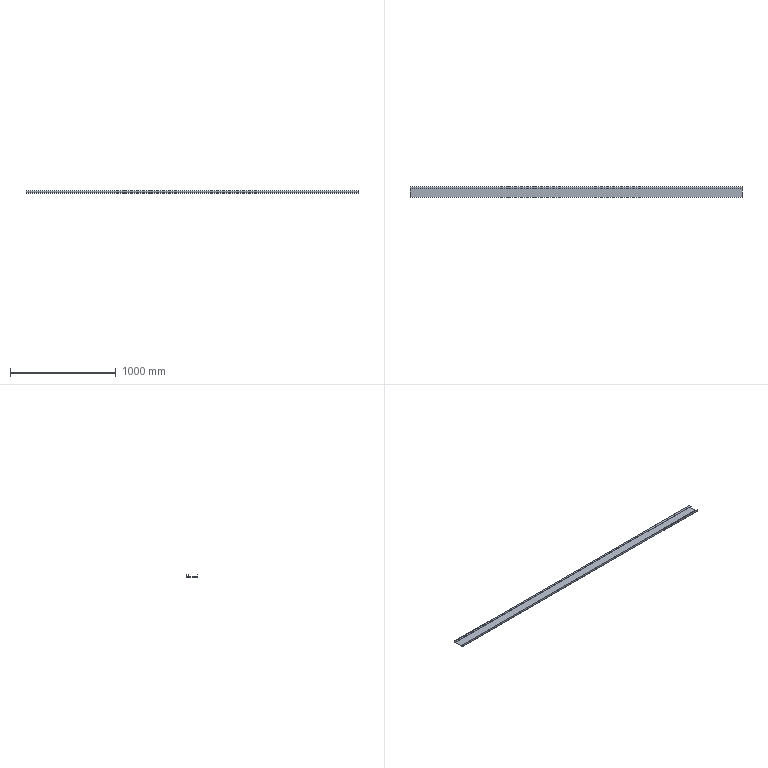Part | STEP file | 电柜护栏2踢脚Plate | 1 solid | 18 faces | box 3145 x 100 x 20 mm | volume 722941 mm3 | plane 12 | cylinder 6 | commonest cylinder face diameters 2 x3 5 x3
STEP:
#1=CARTESIAN_POINT('',(0.,0.,0.));
#2=DIRECTION('',(0.,0.,1.));
#3=DIRECTION('',(1.,0.,0.));
#4=AXIS2_PLACEMENT_3D('',#1,#2,#3);
#5=CARTESIAN_POINT('',(-1572.5,1.5,2.5));
#6=VERTEX_POINT('',#5);
#7=CARTESIAN_POINT('',(-1572.5,1.5,20.));
#8=VERTEX_POINT('',#7);
#9=CARTESIAN_POINT('',(-1572.5,1.5,2.5));
#10=DIRECTION('',(0.,0.,1.));
#11=VECTOR('',#10,1.);
#12=LINE('',#9,#11);
#13=CARTESIAN_POINT('',(1572.5,1.5,2.5));
#14=DIRECTION('',(0.,-1.,0.));
#15=DIRECTION('',(0.,0.,-1.));
#16=AXIS2_PLACEMENT_3D('',#13,#14,#15);
#17=PLANE('',#16);
#18=CARTESIAN_POINT('',(0.,-3145.));
#19=DIRECTION('',(-1.,0.));
#20=VECTOR('',#19,1.);
#21=LINE('',#18,#20);
#22=(GEOMETRIC_REPRESENTATION_CONTEXT(2)PARAMETRIC_REPRESENTATION_CONTEXT()REPRESENTATION_CONTEXT('',''));
#23=DEFINITIONAL_REPRESENTATION('',(#21),#22);
#24=PCURVE('',#17,#23);
#25=CARTESIAN_POINT('',(-1572.5,2.5,2.5));
#26=DIRECTION('',(-1.,0.,0.));
#27=DIRECTION('',(0.,0.,1.));
#28=AXIS2_PLACEMENT_3D('',#25,#26,#27);
#29=PLANE('',#28);
#30=CARTESIAN_POINT('',(0.,-1.));
#31=DIRECTION('',(1.,0.));
#32=VECTOR('',#31,1.);
#33=LINE('',#30,#32);
#34=(GEOMETRIC_REPRESENTATION_CONTEXT(2)PARAMETRIC_REPRESENTATION_CONTEXT()REPRESENTATION_CONTEXT('',''));
#35=DEFINITIONAL_REPRESENTATION('',(#33),#34);
#36=PCURVE('',#29,#35);
#37=SURFACE_CURVE('',#12,(#24,#36),.PCURVE_S1.);
#38=EDGE_CURVE('',#6,#8,#37,.T.);
#39=ORIENTED_EDGE('',*,*,#38,.T.);
#40=CARTESIAN_POINT('',(1572.5,1.5,20.));
#41=VERTEX_POINT('',#40);
#42=CARTESIAN_POINT('',(1572.5,1.5,20.));
#43=DIRECTION('',(-1.,0.,0.));
#44=VECTOR('',#43,1.);
#45=LINE('',#42,#44);
#46=CARTESIAN_POINT('',(-17.5,0.));
#47=DIRECTION('',(0.,-1.));
#48=VECTOR('',#47,1.);
#49=LINE('',#46,#48);
#50=(GEOMETRIC_REPRESENTATION_CONTEXT(2)PARAMETRIC_REPRESENTATION_CONTEXT()REPRESENTATION_CONTEXT('',''));
#51=DEFINITIONAL_REPRESENTATION('',(#49),#50);
#52=PCURVE('',#17,#51);
#53=CARTESIAN_POINT('',(1572.5,0.,20.));
#54=DIRECTION('',(0.,0.,1.));
#55=DIRECTION('',(1.,0.,0.));
#56=AXIS2_PLACEMENT_3D('',#53,#54,#55);
#57=PLANE('',#56);
#58=CARTESIAN_POINT('',(0.,1.5));
#59=DIRECTION('',(-1.,0.));
#60=VECTOR('',#59,1.);
#61=LINE('',#58,#60);
#62=(GEOMETRIC_REPRESENTATION_CONTEXT(2)PARAMETRIC_REPRESENTATION_CONTEXT()REPRESENTATION_CONTEXT('',''));
#63=DEFINITIONAL_REPRESENTATION('',(#61),#62);
#64=PCURVE('',#57,#63);
#65=SURFACE_CURVE('',#45,(#52,#64),.PCURVE_S1.);
#66=EDGE_CURVE('',#41,#8,#65,.T.);
#67=ORIENTED_EDGE('',*,*,#66,.F.);
#68=CARTESIAN_POINT('',(1572.5,1.5,2.5));
#69=VERTEX_POINT('',#68);
#70=CARTESIAN_POINT('',(1572.5,1.5,2.5));
#71=DIRECTION('',(0.,0.,1.));
#72=VECTOR('',#71,1.);
#73=LINE('',#70,#72);
#74=CARTESIAN_POINT('',(0.,0.));
#75=DIRECTION('',(-1.,0.));
#76=VECTOR('',#75,1.);
#77=LINE('',#74,#76);
#78=(GEOMETRIC_REPRESENTATION_CONTEXT(2)PARAMETRIC_REPRESENTATION_CONTEXT()REPRESENTATION_CONTEXT('',''));
#79=DEFINITIONAL_REPRESENTATION('',(#77),#78);
#80=PCURVE('',#17,#79);
#81=CARTESIAN_POINT('',(1572.5,2.5,2.5));
#82=DIRECTION('',(-1.,0.,0.));
#83=DIRECTION('',(0.,0.,1.));
#84=AXIS2_PLACEMENT_3D('',#81,#82,#83);
#85=PLANE('',#84);
#86=CARTESIAN_POINT('',(0.,-1.));
#87=DIRECTION('',(1.,0.));
#88=VECTOR('',#87,1.);
#89=LINE('',#86,#88);
#90=(GEOMETRIC_REPRESENTATION_CONTEXT(2)PARAMETRIC_REPRESENTATION_CONTEXT()REPRESENTATION_CONTEXT('',''));
#91=DEFINITIONAL_REPRESENTATION('',(#89),#90);
#92=PCURVE('',#85,#91);
#93=SURFACE_CURVE('',#73,(#80,#92),.PCURVE_S1.);
#94=EDGE_CURVE('',#69,#41,#93,.T.);
#95=ORIENTED_EDGE('',*,*,#94,.F.);
#96=CARTESIAN_POINT('',(1572.5,1.5,2.5));
#97=DIRECTION('',(-1.,0.,0.));
#98=VECTOR('',#97,1.);
#99=LINE('',#96,#98);
#100=CARTESIAN_POINT('',(0.,0.));
#101=DIRECTION('',(0.,-1.));
#102=VECTOR('',#101,1.);
#103=LINE('',#100,#102);
#104=(GEOMETRIC_REPRESENTATION_CONTEXT(2)PARAMETRIC_REPRESENTATION_CONTEXT()REPRESENTATION_CONTEXT('',''));
#105=DEFINITIONAL_REPRESENTATION('',(#103),#104);
#106=PCURVE('',#17,#105);
#107=CARTESIAN_POINT('',(1572.5,2.5,2.5));
#108=DIRECTION('',(-1.,0.,0.));
#109=DIRECTION('',(0.,0.,1.));
#110=AXIS2_PLACEMENT_3D('',#107,#108,#109);
#111=CYLINDRICAL_SURFACE('',#110,1.);
#112=CARTESIAN_POINT('',(4.712,0.));
#113=DIRECTION('',(0.,1.));
#114=VECTOR('',#113,1.);
#115=LINE('',#112,#114);
#116=(GEOMETRIC_REPRESENTATION_CONTEXT(2)PARAMETRIC_REPRESENTATION_CONTEXT()REPRESENTATION_CONTEXT('',''));
#117=DEFINITIONAL_REPRESENTATION('',(#115),#116);
#118=PCURVE('',#111,#117);
#119=SURFACE_CURVE('',#99,(#106,#118),.PCURVE_S1.);
#120=EDGE_CURVE('',#69,#6,#119,.T.);
#121=ORIENTED_EDGE('',*,*,#120,.T.);
#122=EDGE_LOOP('',(#39,#67,#95,#121));
#123=FACE_BOUND('',#122,.T.);
#124=ADVANCED_FACE('',(#123),#17,.F.);
#125=CARTESIAN_POINT('',(-1572.5,0.,20.));
#126=VERTEX_POINT('',#125);
#127=CARTESIAN_POINT('',(-1572.5,0.,20.));
#128=DIRECTION('',(0.,1.,0.));
#129=VECTOR('',#128,1.);
#130=LINE('',#127,#129);
#131=CARTESIAN_POINT('',(-3145.,0.));
#132=DIRECTION('',(0.,1.));
#133=VECTOR('',#132,1.);
#134=LINE('',#131,#133);
#135=(GEOMETRIC_REPRESENTATION_CONTEXT(2)PARAMETRIC_REPRESENTATION_CONTEXT()REPRESENTATION_CONTEXT('',''));
#136=DEFINITIONAL_REPRESENTATION('',(#134),#135);
#137=PCURVE('',#57,#136);
#138=CARTESIAN_POINT('',(17.5,-2.5));
#139=DIRECTION('',(0.,1.));
#140=VECTOR('',#139,1.);
#141=LINE('',#138,#140);
#142=(GEOMETRIC_REPRESENTATION_CONTEXT(2)PARAMETRIC_REPRESENTATION_CONTEXT()REPRESENTATION_CONTEXT('',''));
#143=DEFINITIONAL_REPRESENTATION('',(#141),#142);
#144=PCURVE('',#29,#143);
#145=SURFACE_CURVE('',#130,(#137,#144),.PCURVE_S1.);
#146=EDGE_CURVE('',#126,#8,#145,.T.);
#147=ORIENTED_EDGE('',*,*,#146,.F.);
#148=CARTESIAN_POINT('',(1572.5,0.,20.));
#149=VERTEX_POINT('',#148);
#150=CARTESIAN_POINT('',(1572.5,0.,20.));
#151=DIRECTION('',(-1.,0.,0.));
#152=VECTOR('',#151,1.);
#153=LINE('',#150,#152);
#154=CARTESIAN_POINT('',(0.,0.));
#155=DIRECTION('',(-1.,0.));
#156=VECTOR('',#155,1.);
#157=LINE('',#154,#156);
#158=(GEOMETRIC_REPRESENTATION_CONTEXT(2)PARAMETRIC_REPRESENTATION_CONTEXT()REPRESENTATION_CONTEXT('',''));
#159=DEFINITIONAL_REPRESENTATION('',(#157),#158);
#160=PCURVE('',#57,#159);
#161=CARTESIAN_POINT('',(1572.5,0.,2.5));
#162=DIRECTION('',(0.,-1.,0.));
#163=DIRECTION('',(0.,0.,-1.));
#164=AXIS2_PLACEMENT_3D('',#161,#162,#163);
#165=PLANE('',#164);
#166=CARTESIAN_POINT('',(-17.5,0.));
#167=DIRECTION('',(0.,-1.));
#168=VECTOR('',#167,1.);
#169=LINE('',#166,#168);
#170=(GEOMETRIC_REPRESENTATION_CONTEXT(2)PARAMETRIC_REPRESENTATION_CONTEXT()REPRESENTATION_CONTEXT('',''));
#171=DEFINITIONAL_REPRESENTATION('',(#169),#170);
#172=PCURVE('',#165,#171);
#173=SURFACE_CURVE('',#153,(#160,#172),.PCURVE_S1.);
#174=EDGE_CURVE('',#149,#126,#173,.T.);
#175=ORIENTED_EDGE('',*,*,#174,.F.);
#176=CARTESIAN_POINT('',(1572.5,0.,20.));
#177=DIRECTION('',(0.,1.,0.));
#178=VECTOR('',#177,1.);
#179=LINE('',#176,#178);
#180=CARTESIAN_POINT('',(0.,0.));
#181=DIRECTION('',(0.,1.));
#182=VECTOR('',#181,1.);
#183=LINE('',#180,#182);
#184=(GEOMETRIC_REPRESENTATION_CONTEXT(2)PARAMETRIC_REPRESENTATION_CONTEXT()REPRESENTATION_CONTEXT('',''));
#185=DEFINITIONAL_REPRESENTATION('',(#183),#184);
#186=PCURVE('',#57,#185);
#187=CARTESIAN_POINT('',(17.5,-2.5));
#188=DIRECTION('',(0.,1.));
#189=VECTOR('',#188,1.);
#190=LINE('',#187,#189);
#191=(GEOMETRIC_REPRESENTATION_CONTEXT(2)PARAMETRIC_REPRESENTATION_CONTEXT()REPRESENTATION_CONTEXT('',''));
#192=DEFINITIONAL_REPRESENTATION('',(#190),#191);
#193=PCURVE('',#85,#192);
#194=SURFACE_CURVE('',#179,(#186,#193),.PCURVE_S1.);
#195=EDGE_CURVE('',#149,#41,#194,.T.);
#196=ORIENTED_EDGE('',*,*,#195,.T.);
#197=ORIENTED_EDGE('',*,*,#66,.T.);
#198=EDGE_LOOP('',(#147,#175,#196,#197));
#199=FACE_BOUND('',#198,.T.);
#200=ADVANCED_FACE('',(#199),#57,.T.);
#201=CARTESIAN_POINT('',(-1572.5,0.,2.5));
#202=VERTEX_POINT('',#201);
#203=CARTESIAN_POINT('',(-1572.5,0.,2.5));
#204=DIRECTION('',(0.,0.,1.));
#205=VECTOR('',#204,1.);
#206=LINE('',#203,#205);
#207=CARTESIAN_POINT('',(0.,-3145.));
#208=DIRECTION('',(-1.,0.));
#209=VECTOR('',#208,1.);
#210=LINE('',#207,#209);
#211=(GEOMETRIC_REPRESENTATION_CONTEXT(2)PARAMETRIC_REPRESENTATION_CONTEXT()REPRESENTATION_CONTEXT('',''));
#212=DEFINITIONAL_REPRESENTATION('',(#210),#211);
#213=PCURVE('',#165,#212);
#214=CARTESIAN_POINT('',(0.,-2.5));
#215=DIRECTION('',(1.,0.));
#216=VECTOR('',#215,1.);
#217=LINE('',#214,#216);
#218=(GEOMETRIC_REPRESENTATION_CONTEXT(2)PARAMETRIC_REPRESENTATION_CONTEXT()REPRESENTATION_CONTEXT('',''));
#219=DEFINITIONAL_REPRESENTATION('',(#217),#218);
#220=PCURVE('',#29,#219);
#221=SURFACE_CURVE('',#206,(#213,#220),.PCURVE_S1.);
#222=EDGE_CURVE('',#202,#126,#221,.T.);
#223=ORIENTED_EDGE('',*,*,#222,.F.);
#224=CARTESIAN_POINT('',(1572.5,0.,2.5));
#225=VERTEX_POINT('',#224);
#226=CARTESIAN_POINT('',(1572.5,0.,2.5));
#227=DIRECTION('',(-1.,0.,0.));
#228=VECTOR('',#227,1.);
#229=LINE('',#226,#228);
#230=CARTESIAN_POINT('',(0.,0.));
#231=DIRECTION('',(0.,-1.));
#232=VECTOR('',#231,1.);
#233=LINE('',#230,#232);
#234=(GEOMETRIC_REPRESENTATION_CONTEXT(2)PARAMETRIC_REPRESENTATION_CONTEXT()REPRESENTATION_CONTEXT('',''));
#235=DEFINITIONAL_REPRESENTATION('',(#233),#234);
#236=PCURVE('',#165,#235);
#237=CARTESIAN_POINT('',(1572.5,2.5,2.5));
#238=DIRECTION('',(-1.,0.,0.));
#239=DIRECTION('',(0.,0.,1.));
#240=AXIS2_PLACEMENT_3D('',#237,#238,#239);
#241=CYLINDRICAL_SURFACE('',#240,2.5);
#242=CARTESIAN_POINT('',(4.712,0.));
#243=DIRECTION('',(0.,1.));
#244=VECTOR('',#243,1.);
#245=LINE('',#242,#244);
#246=(GEOMETRIC_REPRESENTATION_CONTEXT(2)PARAMETRIC_REPRESENTATION_CONTEXT()REPRESENTATION_CONTEXT('',''));
#247=DEFINITIONAL_REPRESENTATION('',(#245),#246);
#248=PCURVE('',#241,#247);
#249=SURFACE_CURVE('',#229,(#236,#248),.PCURVE_S1.);
#250=EDGE_CURVE('',#225,#202,#249,.T.);
#251=ORIENTED_EDGE('',*,*,#250,.F.);
#252=CARTESIAN_POINT('',(1572.5,0.,2.5));
#253=DIRECTION('',(0.,0.,1.));
#254=VECTOR('',#253,1.);
#255=LINE('',#252,#254);
#256=CARTESIAN_POINT('',(0.,0.));
#257=DIRECTION('',(-1.,0.));
#258=VECTOR('',#257,1.);
#259=LINE('',#256,#258);
#260=(GEOMETRIC_REPRESENTATION_CONTEXT(2)PARAMETRIC_REPRESENTATION_CONTEXT()REPRESENTATION_CONTEXT('',''));
#261=DEFINITIONAL_REPRESENTATION('',(#259),#260);
#262=PCURVE('',#165,#261);
#263=CARTESIAN_POINT('',(0.,-2.5));
#264=DIRECTION('',(1.,0.));
#265=VECTOR('',#264,1.);
#266=LINE('',#263,#265);
#267=(GEOMETRIC_REPRESENTATION_CONTEXT(2)PARAMETRIC_REPRESENTATION_CONTEXT()REPRESENTATION_CONTEXT('',''));
#268=DEFINITIONAL_REPRESENTATION('',(#266),#267);
#269=PCURVE('',#85,#268);
#270=SURFACE_CURVE('',#255,(#262,#269),.PCURVE_S1.);
#271=EDGE_CURVE('',#225,#149,#270,.T.);
#272=ORIENTED_EDGE('',*,*,#271,.T.);
#273=ORIENTED_EDGE('',*,*,#174,.T.);
#274=EDGE_LOOP('',(#223,#251,#272,#273));
#275=FACE_BOUND('',#274,.T.);
#276=ADVANCED_FACE('',(#275),#165,.T.);
#277=CARTESIAN_POINT('',(-1572.5,2.5,0.));
#278=VERTEX_POINT('',#277);
#279=CARTESIAN_POINT('',(-1572.5,2.5,2.5));
#280=DIRECTION('',(-1.,0.,0.));
#281=DIRECTION('',(0.,0.,1.));
#282=AXIS2_PLACEMENT_3D('',#279,#280,#281);
#283=CIRCLE('',#282,2.5);
#284=CARTESIAN_POINT('',(0.,3145.));
#285=DIRECTION('',(1.,0.));
#286=VECTOR('',#285,1.);
#287=LINE('',#284,#286);
#288=(GEOMETRIC_REPRESENTATION_CONTEXT(2)PARAMETRIC_REPRESENTATION_CONTEXT()REPRESENTATION_CONTEXT('',''));
#289=DEFINITIONAL_REPRESENTATION('',(#287),#288);
#290=PCURVE('',#241,#289);
#291=CARTESIAN_POINT('',(0.,0.));
#292=DIRECTION('',(1.,0.));
#293=AXIS2_PLACEMENT_2D('',#291,#292);
#294=CIRCLE('',#293,2.5);
#295=(GEOMETRIC_REPRESENTATION_CONTEXT(2)PARAMETRIC_REPRESENTATION_CONTEXT()REPRESENTATION_CONTEXT('',''));
#296=DEFINITIONAL_REPRESENTATION('',(#294),#295);
#297=PCURVE('',#29,#296);
#298=SURFACE_CURVE('',#283,(#290,#297),.PCURVE_S1.);
#299=EDGE_CURVE('',#278,#202,#298,.T.);
#300=ORIENTED_EDGE('',*,*,#299,.F.);
#301=CARTESIAN_POINT('',(1572.5,2.5,0.));
#302=VERTEX_POINT('',#301);
#303=CARTESIAN_POINT('',(1572.5,2.5,0.));
#304=DIRECTION('',(-1.,0.,0.));
#305=VECTOR('',#304,1.);
#306=LINE('',#303,#305);
#307=CARTESIAN_POINT('',(3.142,0.));
#308=DIRECTION('',(0.,1.));
#309=VECTOR('',#308,1.);
#310=LINE('',#307,#309);
#311=(GEOMETRIC_REPRESENTATION_CONTEXT(2)PARAMETRIC_REPRESENTATION_CONTEXT()REPRESENTATION_CONTEXT('',''));
#312=DEFINITIONAL_REPRESENTATION('',(#310),#311);
#313=PCURVE('',#241,#312);
#314=CARTESIAN_POINT('',(1572.5,2.5,0.));
#315=DIRECTION('',(0.,0.,-1.));
#316=DIRECTION('',(-1.,0.,0.));
#317=AXIS2_PLACEMENT_3D('',#314,#315,#316);
#318=PLANE('',#317);
#319=CARTESIAN_POINT('',(0.,0.));
#320=DIRECTION('',(1.,0.));
#321=VECTOR('',#320,1.);
#322=LINE('',#319,#321);
#323=(GEOMETRIC_REPRESENTATION_CONTEXT(2)PARAMETRIC_REPRESENTATION_CONTEXT()REPRESENTATION_CONTEXT('',''));
#324=DEFINITIONAL_REPRESENTATION('',(#322),#323);
#325=PCURVE('',#318,#324);
#326=SURFACE_CURVE('',#306,(#313,#325),.PCURVE_S1.);
#327=EDGE_CURVE('',#302,#278,#326,.T.);
#328=ORIENTED_EDGE('',*,*,#327,.F.);
#329=CARTESIAN_POINT('',(1572.5,2.5,2.5));
#330=DIRECTION('',(-1.,0.,0.));
#331=DIRECTION('',(0.,0.,1.));
#332=AXIS2_PLACEMENT_3D('',#329,#330,#331);
#333=CIRCLE('',#332,2.5);
#334=CARTESIAN_POINT('',(0.,0.));
#335=DIRECTION('',(1.,0.));
#336=VECTOR('',#335,1.);
#337=LINE('',#334,#336);
#338=(GEOMETRIC_REPRESENTATION_CONTEXT(2)PARAMETRIC_REPRESENTATION_CONTEXT()REPRESENTATION_CONTEXT('',''));
#339=DEFINITIONAL_REPRESENTATION('',(#337),#338);
#340=PCURVE('',#241,#339);
#341=CARTESIAN_POINT('',(0.,0.));
#342=DIRECTION('',(1.,0.));
#343=AXIS2_PLACEMENT_2D('',#341,#342);
#344=CIRCLE('',#343,2.5);
#345=(GEOMETRIC_REPRESENTATION_CONTEXT(2)PARAMETRIC_REPRESENTATION_CONTEXT()REPRESENTATION_CONTEXT('',''));
#346=DEFINITIONAL_REPRESENTATION('',(#344),#345);
#347=PCURVE('',#85,#346);
#348=SURFACE_CURVE('',#333,(#340,#347),.PCURVE_S1.);
#349=EDGE_CURVE('',#302,#225,#348,.T.);
#350=ORIENTED_EDGE('',*,*,#349,.T.);
#351=ORIENTED_EDGE('',*,*,#250,.T.);
#352=EDGE_LOOP('',(#300,#328,#350,#351));
#353=FACE_BOUND('',#352,.T.);
#354=ADVANCED_FACE('',(#353),#241,.T.);
#355=CARTESIAN_POINT('',(-1572.5,97.5,0.));
#356=VERTEX_POINT('',#355);
#357=CARTESIAN_POINT('',(-1572.5,2.5,0.));
#358=DIRECTION('',(0.,-1.,0.));
#359=VECTOR('',#358,1.);
#360=LINE('',#357,#359);
#361=CARTESIAN_POINT('',(3145.,0.));
#362=DIRECTION('',(0.,-1.));
#363=VECTOR('',#362,1.);
#364=LINE('',#361,#363);
#365=(GEOMETRIC_REPRESENTATION_CONTEXT(2)PARAMETRIC_REPRESENTATION_CONTEXT()REPRESENTATION_CONTEXT('',''));
#366=DEFINITIONAL_REPRESENTATION('',(#364),#365);
#367=PCURVE('',#318,#366);
#368=CARTESIAN_POINT('',(-2.5,0.));
#369=DIRECTION('',(0.,-1.));
#370=VECTOR('',#369,1.);
#371=LINE('',#368,#370);
#372=(GEOMETRIC_REPRESENTATION_CONTEXT(2)PARAMETRIC_REPRESENTATION_CONTEXT()REPRESENTATION_CONTEXT('',''));
#373=DEFINITIONAL_REPRESENTATION('',(#371),#372);
#374=PCURVE('',#29,#373);
#375=SURFACE_CURVE('',#360,(#367,#374),.PCURVE_S1.);
#376=EDGE_CURVE('',#356,#278,#375,.T.);
#377=ORIENTED_EDGE('',*,*,#376,.F.);
#378=CARTESIAN_POINT('',(1572.5,97.5,0.));
#379=VERTEX_POINT('',#378);
#380=CARTESIAN_POINT('',(1572.5,97.5,0.));
#381=DIRECTION('',(-1.,0.,0.));
#382=VECTOR('',#381,1.);
#383=LINE('',#380,#382);
#384=CARTESIAN_POINT('',(0.,95.));
#385=DIRECTION('',(1.,0.));
#386=VECTOR('',#385,1.);
#387=LINE('',#384,#386);
#388=(GEOMETRIC_REPRESENTATION_CONTEXT(2)PARAMETRIC_REPRESENTATION_CONTEXT()REPRESENTATION_CONTEXT('',''));
#389=DEFINITIONAL_REPRESENTATION('',(#387),#388);
#390=PCURVE('',#318,#389);
#391=CARTESIAN_POINT('',(1572.5,97.5,2.5));
#392=DIRECTION('',(-1.,0.,0.));
#393=DIRECTION('',(0.,0.,1.));
#394=AXIS2_PLACEMENT_3D('',#391,#392,#393);
#395=CYLINDRICAL_SURFACE('',#394,2.5);
#396=CARTESIAN_POINT('',(3.142,0.));
#397=DIRECTION('',(0.,1.));
#398=VECTOR('',#397,1.);
#399=LINE('',#396,#398);
#400=(GEOMETRIC_REPRESENTATION_CONTEXT(2)PARAMETRIC_REPRESENTATION_CONTEXT()REPRESENTATION_CONTEXT('',''));
#401=DEFINITIONAL_REPRESENTATION('',(#399),#400);
#402=PCURVE('',#395,#401);
#403=SURFACE_CURVE('',#383,(#390,#402),.PCURVE_S1.);
#404=EDGE_CURVE('',#379,#356,#403,.T.);
#405=ORIENTED_EDGE('',*,*,#404,.F.);
#406=CARTESIAN_POINT('',(1572.5,2.5,0.));
#407=DIRECTION('',(0.,-1.,0.));
#408=VECTOR('',#407,1.);
#409=LINE('',#406,#408);
#410=CARTESIAN_POINT('',(0.,0.));
#411=DIRECTION('',(0.,-1.));
#412=VECTOR('',#411,1.);
#413=LINE('',#410,#412);
#414=(GEOMETRIC_REPRESENTATION_CONTEXT(2)PARAMETRIC_REPRESENTATION_CONTEXT()REPRESENTATION_CONTEXT('',''));
#415=DEFINITIONAL_REPRESENTATION('',(#413),#414);
#416=PCURVE('',#318,#415);
#417=CARTESIAN_POINT('',(-2.5,0.));
#418=DIRECTION('',(0.,-1.));
#419=VECTOR('',#418,1.);
#420=LINE('',#417,#419);
#421=(GEOMETRIC_REPRESENTATION_CONTEXT(2)PARAMETRIC_REPRESENTATION_CONTEXT()REPRESENTATION_CONTEXT('',''));
#422=DEFINITIONAL_REPRESENTATION('',(#420),#421);
#423=PCURVE('',#85,#422);
#424=SURFACE_CURVE('',#409,(#416,#423),.PCURVE_S1.);
#425=EDGE_CURVE('',#379,#302,#424,.T.);
#426=ORIENTED_EDGE('',*,*,#425,.T.);
#427=ORIENTED_EDGE('',*,*,#327,.T.);
#428=EDGE_LOOP('',(#377,#405,#426,#427));
#429=FACE_BOUND('',#428,.T.);
#430=ADVANCED_FACE('',(#429),#318,.T.);
#431=CARTESIAN_POINT('',(-1572.5,100.,2.5));
#432=VERTEX_POINT('',#431);
#433=CARTESIAN_POINT('',(-1572.5,97.5,2.5));
#434=DIRECTION('',(-1.,0.,0.));
#435=DIRECTION('',(0.,0.,-1.));
#436=AXIS2_PLACEMENT_3D('',#433,#434,#435);
#437=CIRCLE('',#436,2.5);
#438=CARTESIAN_POINT('',(-3.142,3145.));
#439=DIRECTION('',(1.,0.));
#440=VECTOR('',#439,1.);
#441=LINE('',#438,#440);
#442=(GEOMETRIC_REPRESENTATION_CONTEXT(2)PARAMETRIC_REPRESENTATION_CONTEXT()REPRESENTATION_CONTEXT('',''));
#443=DEFINITIONAL_REPRESENTATION('',(#441),#442);
#444=PCURVE('',#395,#443);
#445=CARTESIAN_POINT('',(0.,95.));
#446=DIRECTION('',(-1.,0.));
#447=AXIS2_PLACEMENT_2D('',#445,#446);
#448=CIRCLE('',#447,2.5);
#449=(GEOMETRIC_REPRESENTATION_CONTEXT(2)PARAMETRIC_REPRESENTATION_CONTEXT()REPRESENTATION_CONTEXT('',''));
#450=DEFINITIONAL_REPRESENTATION('',(#448),#449);
#451=PCURVE('',#29,#450);
#452=SURFACE_CURVE('',#437,(#444,#451),.PCURVE_S1.);
#453=EDGE_CURVE('',#432,#356,#452,.T.);
#454=ORIENTED_EDGE('',*,*,#453,.F.);
#455=CARTESIAN_POINT('',(1572.5,100.,2.5));
#456=VERTEX_POINT('',#455);
#457=CARTESIAN_POINT('',(1572.5,100.,2.5));
#458=DIRECTION('',(-1.,0.,0.));
#459=VECTOR('',#458,1.);
#460=LINE('',#457,#459);
#461=CARTESIAN_POINT('',(1.571,0.));
#462=DIRECTION('',(0.,1.));
#463=VECTOR('',#462,1.);
#464=LINE('',#461,#463);
#465=(GEOMETRIC_REPRESENTATION_CONTEXT(2)PARAMETRIC_REPRESENTATION_CONTEXT()REPRESENTATION_CONTEXT('',''));
#466=DEFINITIONAL_REPRESENTATION('',(#464),#465);
#467=PCURVE('',#395,#466);
#468=CARTESIAN_POINT('',(1572.5,100.,2.5));
#469=DIRECTION('',(0.,1.,0.));
#470=DIRECTION('',(0.,0.,1.));
#471=AXIS2_PLACEMENT_3D('',#468,#469,#470);
#472=PLANE('',#471);
#473=CARTESIAN_POINT('',(0.,0.));
#474=DIRECTION('',(0.,-1.));
#475=VECTOR('',#474,1.);
#476=LINE('',#473,#475);
#477=(GEOMETRIC_REPRESENTATION_CONTEXT(2)PARAMETRIC_REPRESENTATION_CONTEXT()REPRESENTATION_CONTEXT('',''));
#478=DEFINITIONAL_REPRESENTATION('',(#476),#477);
#479=PCURVE('',#472,#478);
#480=SURFACE_CURVE('',#460,(#467,#479),.PCURVE_S1.);
#481=EDGE_CURVE('',#456,#432,#480,.T.);
#482=ORIENTED_EDGE('',*,*,#481,.F.);
#483=CARTESIAN_POINT('',(1572.5,97.5,2.5));
#484=DIRECTION('',(-1.,0.,0.));
#485=DIRECTION('',(0.,0.,-1.));
#486=AXIS2_PLACEMENT_3D('',#483,#484,#485);
#487=CIRCLE('',#486,2.5);
#488=CARTESIAN_POINT('',(-3.142,0.));
#489=DIRECTION('',(1.,0.));
#490=VECTOR('',#489,1.);
#491=LINE('',#488,#490);
#492=(GEOMETRIC_REPRESENTATION_CONTEXT(2)PARAMETRIC_REPRESENTATION_CONTEXT()REPRESENTATION_CONTEXT('',''));
#493=DEFINITIONAL_REPRESENTATION('',(#491),#492);
#494=PCURVE('',#395,#493);
#495=CARTESIAN_POINT('',(0.,95.));
#496=DIRECTION('',(-1.,0.));
#497=AXIS2_PLACEMENT_2D('',#495,#496);
#498=CIRCLE('',#497,2.5);
#499=(GEOMETRIC_REPRESENTATION_CONTEXT(2)PARAMETRIC_REPRESENTATION_CONTEXT()REPRESENTATION_CONTEXT('',''));
#500=DEFINITIONAL_REPRESENTATION('',(#498),#499);
#501=PCURVE('',#85,#500);
#502=SURFACE_CURVE('',#487,(#494,#501),.PCURVE_S1.);
#503=EDGE_CURVE('',#456,#379,#502,.T.);
#504=ORIENTED_EDGE('',*,*,#503,.T.);
#505=ORIENTED_EDGE('',*,*,#404,.T.);
#506=EDGE_LOOP('',(#454,#482,#504,#505));
#507=FACE_BOUND('',#506,.T.);
#508=ADVANCED_FACE('',(#507),#395,.T.);
#509=CARTESIAN_POINT('',(-1572.5,100.,17.5));
#510=VERTEX_POINT('',#509);
#511=CARTESIAN_POINT('',(-1572.5,100.,2.5));
#512=DIRECTION('',(0.,0.,-1.));
#513=VECTOR('',#512,1.);
#514=LINE('',#511,#513);
#515=CARTESIAN_POINT('',(0.,-3145.));
#516=DIRECTION('',(-1.,0.));
#517=VECTOR('',#516,1.);
#518=LINE('',#515,#517);
#519=(GEOMETRIC_REPRESENTATION_CONTEXT(2)PARAMETRIC_REPRESENTATION_CONTEXT()REPRESENTATION_CONTEXT('',''));
#520=DEFINITIONAL_REPRESENTATION('',(#518),#519);
#521=PCURVE('',#472,#520);
#522=CARTESIAN_POINT('',(0.,97.5));
#523=DIRECTION('',(-1.,0.));
#524=VECTOR('',#523,1.);
#525=LINE('',#522,#524);
#526=(GEOMETRIC_REPRESENTATION_CONTEXT(2)PARAMETRIC_REPRESENTATION_CONTEXT()REPRESENTATION_CONTEXT('',''));
#527=DEFINITIONAL_REPRESENTATION('',(#525),#526);
#528=PCURVE('',#29,#527);
#529=SURFACE_CURVE('',#514,(#521,#528),.PCURVE_S1.);
#530=EDGE_CURVE('',#510,#432,#529,.T.);
#531=ORIENTED_EDGE('',*,*,#530,.F.);
#532=CARTESIAN_POINT('',(1572.5,100.,17.5));
#533=VERTEX_POINT('',#532);
#534=CARTESIAN_POINT('',(1572.5,100.,17.5));
#535=DIRECTION('',(-1.,0.,0.));
#536=VECTOR('',#535,1.);
#537=LINE('',#534,#536);
#538=CARTESIAN_POINT('',(15.,0.));
#539=DIRECTION('',(0.,-1.));
#540=VECTOR('',#539,1.);
#541=LINE('',#538,#540);
#542=(GEOMETRIC_REPRESENTATION_CONTEXT(2)PARAMETRIC_REPRESENTATION_CONTEXT()REPRESENTATION_CONTEXT('',''));
#543=DEFINITIONAL_REPRESENTATION('',(#541),#542);
#544=PCURVE('',#472,#543);
#545=CARTESIAN_POINT('',(1572.5,97.5,17.5));
#546=DIRECTION('',(-1.,0.,0.));
#547=DIRECTION('',(0.,0.,1.));
#548=AXIS2_PLACEMENT_3D('',#545,#546,#547);
#549=CYLINDRICAL_SURFACE('',#548,2.5);
#550=CARTESIAN_POINT('',(1.571,0.));
#551=DIRECTION('',(0.,1.));
#552=VECTOR('',#551,1.);
#553=LINE('',#550,#552);
#554=(GEOMETRIC_REPRESENTATION_CONTEXT(2)PARAMETRIC_REPRESENTATION_CONTEXT()REPRESENTATION_CONTEXT('',''));
#555=DEFINITIONAL_REPRESENTATION('',(#553),#554);
#556=PCURVE('',#549,#555);
#557=SURFACE_CURVE('',#537,(#544,#556),.PCURVE_S1.);
#558=EDGE_CURVE('',#533,#510,#557,.T.);
#559=ORIENTED_EDGE('',*,*,#558,.F.);
#560=CARTESIAN_POINT('',(1572.5,100.,2.5));
#561=DIRECTION('',(0.,0.,-1.));
#562=VECTOR('',#561,1.);
#563=LINE('',#560,#562);
#564=CARTESIAN_POINT('',(0.,0.));
#565=DIRECTION('',(-1.,0.));
#566=VECTOR('',#565,1.);
#567=LINE('',#564,#566);
#568=(GEOMETRIC_REPRESENTATION_CONTEXT(2)PARAMETRIC_REPRESENTATION_CONTEXT()REPRESENTATION_CONTEXT('',''));
#569=DEFINITIONAL_REPRESENTATION('',(#567),#568);
#570=PCURVE('',#472,#569);
#571=CARTESIAN_POINT('',(0.,97.5));
#572=DIRECTION('',(-1.,0.));
#573=VECTOR('',#572,1.);
#574=LINE('',#571,#573);
#575=(GEOMETRIC_REPRESENTATION_CONTEXT(2)PARAMETRIC_REPRESENTATION_CONTEXT()REPRESENTATION_CONTEXT('',''));
#576=DEFINITIONAL_REPRESENTATION('',(#574),#575);
#577=PCURVE('',#85,#576);
#578=SURFACE_CURVE('',#563,(#570,#577),.PCURVE_S1.);
#579=EDGE_CURVE('',#533,#456,#578,.T.);
#580=ORIENTED_EDGE('',*,*,#579,.T.);
#581=ORIENTED_EDGE('',*,*,#481,.T.);
#582=EDGE_LOOP('',(#531,#559,#580,#581));
#583=FACE_BOUND('',#582,.T.);
#584=ADVANCED_FACE('',(#583),#472,.T.);
#585=CARTESIAN_POINT('',(-1572.5,97.5,20.));
#586=VERTEX_POINT('',#585);
#587=CARTESIAN_POINT('',(-1572.5,97.5,17.5));
#588=DIRECTION('',(-1.,0.,0.));
#589=DIRECTION('',(0.,0.,-1.));
#590=AXIS2_PLACEMENT_3D('',#587,#588,#589);
#591=CIRCLE('',#590,2.5);
#592=CARTESIAN_POINT('',(-3.142,3145.));
#593=DIRECTION('',(1.,0.));
#594=VECTOR('',#593,1.);
#595=LINE('',#592,#594);
#596=(GEOMETRIC_REPRESENTATION_CONTEXT(2)PARAMETRIC_REPRESENTATION_CONTEXT()REPRESENTATION_CONTEXT('',''));
#597=DEFINITIONAL_REPRESENTATION('',(#595),#596);
#598=PCURVE('',#549,#597);
#599=CARTESIAN_POINT('',(15.,95.));
#600=DIRECTION('',(-1.,0.));
#601=AXIS2_PLACEMENT_2D('',#599,#600);
#602=CIRCLE('',#601,2.5);
#603=(GEOMETRIC_REPRESENTATION_CONTEXT(2)PARAMETRIC_REPRESENTATION_CONTEXT()REPRESENTATION_CONTEXT('',''));
#604=DEFINITIONAL_REPRESENTATION('',(#602),#603);
#605=PCURVE('',#29,#604);
#606=SURFACE_CURVE('',#591,(#598,#605),.PCURVE_S1.);
#607=EDGE_CURVE('',#586,#510,#606,.T.);
#608=ORIENTED_EDGE('',*,*,#607,.F.);
#609=CARTESIAN_POINT('',(1572.5,97.5,20.));
#610=VERTEX_POINT('',#609);
#611=CARTESIAN_POINT('',(1572.5,97.5,20.));
#612=DIRECTION('',(-1.,0.,0.));
#613=VECTOR('',#612,1.);
#614=LINE('',#611,#613);
#615=CARTESIAN_POINT('',(0.,0.));
#616=DIRECTION('',(0.,1.));
#617=VECTOR('',#616,1.);
#618=LINE('',#615,#617);
#619=(GEOMETRIC_REPRESENTATION_CONTEXT(2)PARAMETRIC_REPRESENTATION_CONTEXT()REPRESENTATION_CONTEXT('',''));
#620=DEFINITIONAL_REPRESENTATION('',(#618),#619);
#621=PCURVE('',#549,#620);
#622=CARTESIAN_POINT('',(1572.5,97.5,20.));
#623=DIRECTION('',(0.,0.,1.));
#624=DIRECTION('',(1.,0.,0.));
#625=AXIS2_PLACEMENT_3D('',#622,#623,#624);
#626=PLANE('',#625);
#627=CARTESIAN_POINT('',(0.,0.));
#628=DIRECTION('',(-1.,0.));
#629=VECTOR('',#628,1.);
#630=LINE('',#627,#629);
#631=(GEOMETRIC_REPRESENTATION_CONTEXT(2)PARAMETRIC_REPRESENTATION_CONTEXT()REPRESENTATION_CONTEXT('',''));
#632=DEFINITIONAL_REPRESENTATION('',(#630),#631);
#633=PCURVE('',#626,#632);
#634=SURFACE_CURVE('',#614,(#621,#633),.PCURVE_S1.);
#635=EDGE_CURVE('',#610,#586,#634,.T.);
#636=ORIENTED_EDGE('',*,*,#635,.F.);
#637=CARTESIAN_POINT('',(1572.5,97.5,17.5));
#638=DIRECTION('',(-1.,0.,0.));
#639=DIRECTION('',(0.,0.,-1.));
#640=AXIS2_PLACEMENT_3D('',#637,#638,#639);
#641=CIRCLE('',#640,2.5);
#642=CARTESIAN_POINT('',(-3.142,0.));
#643=DIRECTION('',(1.,0.));
#644=VECTOR('',#643,1.);
#645=LINE('',#642,#644);
#646=(GEOMETRIC_REPRESENTATION_CONTEXT(2)PARAMETRIC_REPRESENTATION_CONTEXT()REPRESENTATION_CONTEXT('',''));
#647=DEFINITIONAL_REPRESENTATION('',(#645),#646);
#648=PCURVE('',#549,#647);
#649=CARTESIAN_POINT('',(15.,95.));
#650=DIRECTION('',(-1.,0.));
#651=AXIS2_PLACEMENT_2D('',#649,#650);
#652=CIRCLE('',#651,2.5);
#653=(GEOMETRIC_REPRESENTATION_CONTEXT(2)PARAMETRIC_REPRESENTATION_CONTEXT()REPRESENTATION_CONTEXT('',''));
#654=DEFINITIONAL_REPRESENTATION('',(#652),#653);
#655=PCURVE('',#85,#654);
#656=SURFACE_CURVE('',#641,(#648,#655),.PCURVE_S1.);
#657=EDGE_CURVE('',#610,#533,#656,.T.);
#658=ORIENTED_EDGE('',*,*,#657,.T.);
#659=ORIENTED_EDGE('',*,*,#558,.T.);
#660=EDGE_LOOP('',(#608,#636,#658,#659));
#661=FACE_BOUND('',#660,.T.);
#662=ADVANCED_FACE('',(#661),#549,.T.);
#663=CARTESIAN_POINT('',(-1572.5,80.,20.));
#664=VERTEX_POINT('',#663);
#665=CARTESIAN_POINT('',(-1572.5,97.5,20.));
#666=DIRECTION('',(0.,1.,0.));
#667=VECTOR('',#666,1.);
#668=LINE('',#665,#667);
#669=CARTESIAN_POINT('',(-3145.,0.));
#670=DIRECTION('',(0.,1.));
#671=VECTOR('',#670,1.);
#672=LINE('',#669,#671);
#673=(GEOMETRIC_REPRESENTATION_CONTEXT(2)PARAMETRIC_REPRESENTATION_CONTEXT()REPRESENTATION_CONTEXT('',''));
#674=DEFINITIONAL_REPRESENTATION('',(#672),#673);
#675=PCURVE('',#626,#674);
#676=CARTESIAN_POINT('',(17.5,95.));
#677=DIRECTION('',(0.,1.));
#678=VECTOR('',#677,1.);
#679=LINE('',#676,#678);
#680=(GEOMETRIC_REPRESENTATION_CONTEXT(2)PARAMETRIC_REPRESENTATION_CONTEXT()REPRESENTATION_CONTEXT('',''));
#681=DEFINITIONAL_REPRESENTATION('',(#679),#680);
#682=PCURVE('',#29,#681);
#683=SURFACE_CURVE('',#668,(#675,#682),.PCURVE_S1.);
#684=EDGE_CURVE('',#664,#586,#683,.T.);
#685=ORIENTED_EDGE('',*,*,#684,.F.);
#686=CARTESIAN_POINT('',(1572.5,80.,20.));
#687=VERTEX_POINT('',#686);
#688=CARTESIAN_POINT('',(1572.5,80.,20.));
#689=DIRECTION('',(-1.,0.,0.));
#690=VECTOR('',#689,1.);
#691=LINE('',#688,#690);
#692=CARTESIAN_POINT('',(0.,-17.5));
#693=DIRECTION('',(-1.,0.));
#694=VECTOR('',#693,1.);
#695=LINE('',#692,#694);
#696=(GEOMETRIC_REPRESENTATION_CONTEXT(2)PARAMETRIC_REPRESENTATION_CONTEXT()REPRESENTATION_CONTEXT('',''));
#697=DEFINITIONAL_REPRESENTATION('',(#695),#696);
#698=PCURVE('',#626,#697);
#699=CARTESIAN_POINT('',(1572.5,80.,18.5));
#700=DIRECTION('',(0.,-1.,0.));
#701=DIRECTION('',(0.,0.,-1.));
#702=AXIS2_PLACEMENT_3D('',#699,#700,#701);
#703=PLANE('',#702);
#704=CARTESIAN_POINT('',(-1.5,0.));
#705=DIRECTION('',(0.,-1.));
#706=VECTOR('',#705,1.);
#707=LINE('',#704,#706);
#708=(GEOMETRIC_REPRESENTATION_CONTEXT(2)PARAMETRIC_REPRESENTATION_CONTEXT()REPRESENTATION_CONTEXT('',''));
#709=DEFINITIONAL_REPRESENTATION('',(#707),#708);
#710=PCURVE('',#703,#709);
#711=SURFACE_CURVE('',#691,(#698,#710),.PCURVE_S1.);
#712=EDGE_CURVE('',#687,#664,#711,.T.);
#713=ORIENTED_EDGE('',*,*,#712,.F.);
#714=CARTESIAN_POINT('',(1572.5,97.5,20.));
#715=DIRECTION('',(0.,1.,0.));
#716=VECTOR('',#715,1.);
#717=LINE('',#714,#716);
#718=CARTESIAN_POINT('',(0.,0.));
#719=DIRECTION('',(0.,1.));
#720=VECTOR('',#719,1.);
#721=LINE('',#718,#720);
#722=(GEOMETRIC_REPRESENTATION_CONTEXT(2)PARAMETRIC_REPRESENTATION_CONTEXT()REPRESENTATION_CONTEXT('',''));
#723=DEFINITIONAL_REPRESENTATION('',(#721),#722);
#724=PCURVE('',#626,#723);
#725=CARTESIAN_POINT('',(17.5,95.));
#726=DIRECTION('',(0.,1.));
#727=VECTOR('',#726,1.);
#728=LINE('',#725,#727);
#729=(GEOMETRIC_REPRESENTATION_CONTEXT(2)PARAMETRIC_REPRESENTATION_CONTEXT()REPRESENTATION_CONTEXT('',''));
#730=DEFINITIONAL_REPRESENTATION('',(#728),#729);
#731=PCURVE('',#85,#730);
#732=SURFACE_CURVE('',#717,(#724,#731),.PCURVE_S1.);
#733=EDGE_CURVE('',#687,#610,#732,.T.);
#734=ORIENTED_EDGE('',*,*,#733,.T.);
#735=ORIENTED_EDGE('',*,*,#635,.T.);
#736=EDGE_LOOP('',(#685,#713,#734,#735));
#737=FACE_BOUND('',#736,.T.);
#738=ADVANCED_FACE('',(#737),#626,.T.);
#739=CARTESIAN_POINT('',(-1572.5,80.,18.5));
#740=VERTEX_POINT('',#739);
#741=CARTESIAN_POINT('',(-1572.5,80.,18.5));
#742=DIRECTION('',(0.,0.,1.));
#743=VECTOR('',#742,1.);
#744=LINE('',#741,#743);
#745=CARTESIAN_POINT('',(0.,-3145.));
#746=DIRECTION('',(-1.,0.));
#747=VECTOR('',#746,1.);
#748=LINE('',#745,#747);
#749=(GEOMETRIC_REPRESENTATION_CONTEXT(2)PARAMETRIC_REPRESENTATION_CONTEXT()REPRESENTATION_CONTEXT('',''));
#750=DEFINITIONAL_REPRESENTATION('',(#748),#749);
#751=PCURVE('',#703,#750);
#752=CARTESIAN_POINT('',(16.,77.5));
#753=DIRECTION('',(1.,0.));
#754=VECTOR('',#753,1.);
#755=LINE('',#752,#754);
#756=(GEOMETRIC_REPRESENTATION_CONTEXT(2)PARAMETRIC_REPRESENTATION_CONTEXT()REPRESENTATION_CONTEXT('',''));
#757=DEFINITIONAL_REPRESENTATION('',(#755),#756);
#758=PCURVE('',#29,#757);
#759=SURFACE_CURVE('',#744,(#751,#758),.PCURVE_S1.);
#760=EDGE_CURVE('',#740,#664,#759,.T.);
#761=ORIENTED_EDGE('',*,*,#760,.F.);
#762=CARTESIAN_POINT('',(1572.5,80.,18.5));
#763=VERTEX_POINT('',#762);
#764=CARTESIAN_POINT('',(1572.5,80.,18.5));
#765=DIRECTION('',(-1.,0.,0.));
#766=VECTOR('',#765,1.);
#767=LINE('',#764,#766);
#768=CARTESIAN_POINT('',(0.,0.));
#769=DIRECTION('',(0.,-1.));
#770=VECTOR('',#769,1.);
#771=LINE('',#768,#770);
#772=(GEOMETRIC_REPRESENTATION_CONTEXT(2)PARAMETRIC_REPRESENTATION_CONTEXT()REPRESENTATION_CONTEXT('',''));
#773=DEFINITIONAL_REPRESENTATION('',(#771),#772);
#774=PCURVE('',#703,#773);
#775=CARTESIAN_POINT('',(1572.5,97.5,18.5));
#776=DIRECTION('',(0.,0.,1.));
#777=DIRECTION('',(1.,0.,0.));
#778=AXIS2_PLACEMENT_3D('',#775,#776,#777);
#779=PLANE('',#778);
#780=CARTESIAN_POINT('',(0.,-17.5));
#781=DIRECTION('',(-1.,0.));
#782=VECTOR('',#781,1.);
#783=LINE('',#780,#782);
#784=(GEOMETRIC_REPRESENTATION_CONTEXT(2)PARAMETRIC_REPRESENTATION_CONTEXT()REPRESENTATION_CONTEXT('',''));
#785=DEFINITIONAL_REPRESENTATION('',(#783),#784);
#786=PCURVE('',#779,#785);
#787=SURFACE_CURVE('',#767,(#774,#786),.PCURVE_S1.);
#788=EDGE_CURVE('',#763,#740,#787,.T.);
#789=ORIENTED_EDGE('',*,*,#788,.F.);
#790=CARTESIAN_POINT('',(1572.5,80.,18.5));
#791=DIRECTION('',(0.,0.,1.));
#792=VECTOR('',#791,1.);
#793=LINE('',#790,#792);
#794=CARTESIAN_POINT('',(0.,0.));
#795=DIRECTION('',(-1.,0.));
#796=VECTOR('',#795,1.);
#797=LINE('',#794,#796);
#798=(GEOMETRIC_REPRESENTATION_CONTEXT(2)PARAMETRIC_REPRESENTATION_CONTEXT()REPRESENTATION_CONTEXT('',''));
#799=DEFINITIONAL_REPRESENTATION('',(#797),#798);
#800=PCURVE('',#703,#799);
#801=CARTESIAN_POINT('',(16.,77.5));
#802=DIRECTION('',(1.,0.));
#803=VECTOR('',#802,1.);
#804=LINE('',#801,#803);
#805=(GEOMETRIC_REPRESENTATION_CONTEXT(2)PARAMETRIC_REPRESENTATION_CONTEXT()REPRESENTATION_CONTEXT('',''));
#806=DEFINITIONAL_REPRESENTATION('',(#804),#805);
#807=PCURVE('',#85,#806);
#808=SURFACE_CURVE('',#793,(#800,#807),.PCURVE_S1.);
#809=EDGE_CURVE('',#763,#687,#808,.T.);
#810=ORIENTED_EDGE('',*,*,#809,.T.);
#811=ORIENTED_EDGE('',*,*,#712,.T.);
#812=EDGE_LOOP('',(#761,#789,#810,#811));
#813=FACE_BOUND('',#812,.T.);
#814=ADVANCED_FACE('',(#813),#703,.T.);
#815=CARTESIAN_POINT('',(-1572.5,97.5,18.5));
#816=VERTEX_POINT('',#815);
#817=CARTESIAN_POINT('',(-1572.5,97.5,18.5));
#818=DIRECTION('',(0.,1.,0.));
#819=VECTOR('',#818,1.);
#820=LINE('',#817,#819);
#821=CARTESIAN_POINT('',(-3145.,0.));
#822=DIRECTION('',(0.,1.));
#823=VECTOR('',#822,1.);
#824=LINE('',#821,#823);
#825=(GEOMETRIC_REPRESENTATION_CONTEXT(2)PARAMETRIC_REPRESENTATION_CONTEXT()REPRESENTATION_CONTEXT('',''));
#826=DEFINITIONAL_REPRESENTATION('',(#824),#825);
#827=PCURVE('',#779,#826);
#828=CARTESIAN_POINT('',(16.,95.));
#829=DIRECTION('',(0.,1.));
#830=VECTOR('',#829,1.);
#831=LINE('',#828,#830);
#832=(GEOMETRIC_REPRESENTATION_CONTEXT(2)PARAMETRIC_REPRESENTATION_CONTEXT()REPRESENTATION_CONTEXT('',''));
#833=DEFINITIONAL_REPRESENTATION('',(#831),#832);
#834=PCURVE('',#29,#833);
#835=SURFACE_CURVE('',#820,(#827,#834),.PCURVE_S1.);
#836=EDGE_CURVE('',#740,#816,#835,.T.);
#837=ORIENTED_EDGE('',*,*,#836,.T.);
#838=CARTESIAN_POINT('',(1572.5,97.5,18.5));
#839=VERTEX_POINT('',#838);
#840=CARTESIAN_POINT('',(1572.5,97.5,18.5));
#841=DIRECTION('',(-1.,0.,0.));
#842=VECTOR('',#841,1.);
#843=LINE('',#840,#842);
#844=CARTESIAN_POINT('',(0.,0.));
#845=DIRECTION('',(-1.,0.));
#846=VECTOR('',#845,1.);
#847=LINE('',#844,#846);
#848=(GEOMETRIC_REPRESENTATION_CONTEXT(2)PARAMETRIC_REPRESENTATION_CONTEXT()REPRESENTATION_CONTEXT('',''));
#849=DEFINITIONAL_REPRESENTATION('',(#847),#848);
#850=PCURVE('',#779,#849);
#851=CARTESIAN_POINT('',(1572.5,97.5,17.5));
#852=DIRECTION('',(-1.,0.,0.));
#853=DIRECTION('',(0.,0.,1.));
#854=AXIS2_PLACEMENT_3D('',#851,#852,#853);
#855=CYLINDRICAL_SURFACE('',#854,1.);
#856=CARTESIAN_POINT('',(0.,0.));
#857=DIRECTION('',(0.,1.));
#858=VECTOR('',#857,1.);
#859=LINE('',#856,#858);
#860=(GEOMETRIC_REPRESENTATION_CONTEXT(2)PARAMETRIC_REPRESENTATION_CONTEXT()REPRESENTATION_CONTEXT('',''));
#861=DEFINITIONAL_REPRESENTATION('',(#859),#860);
#862=PCURVE('',#855,#861);
#863=SURFACE_CURVE('',#843,(#850,#862),.PCURVE_S1.);
#864=EDGE_CURVE('',#839,#816,#863,.T.);
#865=ORIENTED_EDGE('',*,*,#864,.F.);
#866=CARTESIAN_POINT('',(1572.5,97.5,18.5));
#867=DIRECTION('',(0.,1.,0.));
#868=VECTOR('',#867,1.);
#869=LINE('',#866,#868);
#870=CARTESIAN_POINT('',(0.,0.));
#871=DIRECTION('',(0.,1.));
#872=VECTOR('',#871,1.);
#873=LINE('',#870,#872);
#874=(GEOMETRIC_REPRESENTATION_CONTEXT(2)PARAMETRIC_REPRESENTATION_CONTEXT()REPRESENTATION_CONTEXT('',''));
#875=DEFINITIONAL_REPRESENTATION('',(#873),#874);
#876=PCURVE('',#779,#875);
#877=CARTESIAN_POINT('',(16.,95.));
#878=DIRECTION('',(0.,1.));
#879=VECTOR('',#878,1.);
#880=LINE('',#877,#879);
#881=(GEOMETRIC_REPRESENTATION_CONTEXT(2)PARAMETRIC_REPRESENTATION_CONTEXT()REPRESENTATION_CONTEXT('',''));
#882=DEFINITIONAL_REPRESENTATION('',(#880),#881);
#883=PCURVE('',#85,#882);
#884=SURFACE_CURVE('',#869,(#876,#883),.PCURVE_S1.);
#885=EDGE_CURVE('',#763,#839,#884,.T.);
#886=ORIENTED_EDGE('',*,*,#885,.F.);
#887=ORIENTED_EDGE('',*,*,#788,.T.);
#888=EDGE_LOOP('',(#837,#865,#886,#887));
#889=FACE_BOUND('',#888,.T.);
#890=ADVANCED_FACE('',(#889),#779,.F.);
#891=ORIENTED_EDGE('',*,*,#864,.F.);
#892=CARTESIAN_POINT('',(1572.5,98.5,17.5));
#893=VERTEX_POINT('',#892);
#894=CARTESIAN_POINT('',(1572.5,97.5,17.5));
#895=DIRECTION('',(-1.,0.,0.));
#896=DIRECTION('',(0.,0.,-1.));
#897=AXIS2_PLACEMENT_3D('',#894,#895,#896);
#898=CIRCLE('',#897,1.);
#899=CARTESIAN_POINT('',(-3.142,0.));
#900=DIRECTION('',(1.,0.));
#901=VECTOR('',#900,1.);
#902=LINE('',#899,#901);
#903=(GEOMETRIC_REPRESENTATION_CONTEXT(2)PARAMETRIC_REPRESENTATION_CONTEXT()REPRESENTATION_CONTEXT('',''));
#904=DEFINITIONAL_REPRESENTATION('',(#902),#903);
#905=PCURVE('',#855,#904);
#906=CARTESIAN_POINT('',(15.,95.));
#907=DIRECTION('',(-1.,0.));
#908=AXIS2_PLACEMENT_2D('',#906,#907);
#909=CIRCLE('',#908,1.);
#910=(GEOMETRIC_REPRESENTATION_CONTEXT(2)PARAMETRIC_REPRESENTATION_CONTEXT()REPRESENTATION_CONTEXT('',''));
#911=DEFINITIONAL_REPRESENTATION('',(#909),#910);
#912=PCURVE('',#85,#911);
#913=SURFACE_CURVE('',#898,(#905,#912),.PCURVE_S1.);
#914=EDGE_CURVE('',#839,#893,#913,.T.);
#915=ORIENTED_EDGE('',*,*,#914,.T.);
#916=CARTESIAN_POINT('',(-1572.5,98.5,17.5));
#917=VERTEX_POINT('',#916);
#918=CARTESIAN_POINT('',(1572.5,98.5,17.5));
#919=DIRECTION('',(-1.,0.,0.));
#920=VECTOR('',#919,1.);
#921=LINE('',#918,#920);
#922=CARTESIAN_POINT('',(1.571,0.));
#923=DIRECTION('',(0.,1.));
#924=VECTOR('',#923,1.);
#925=LINE('',#922,#924);
#926=(GEOMETRIC_REPRESENTATION_CONTEXT(2)PARAMETRIC_REPRESENTATION_CONTEXT()REPRESENTATION_CONTEXT('',''));
#927=DEFINITIONAL_REPRESENTATION('',(#925),#926);
#928=PCURVE('',#855,#927);
#929=CARTESIAN_POINT('',(1572.5,98.5,2.5));
#930=DIRECTION('',(0.,1.,0.));
#931=DIRECTION('',(0.,0.,1.));
#932=AXIS2_PLACEMENT_3D('',#929,#930,#931);
#933=PLANE('',#932);
#934=CARTESIAN_POINT('',(15.,0.));
#935=DIRECTION('',(0.,-1.));
#936=VECTOR('',#935,1.);
#937=LINE('',#934,#936);
#938=(GEOMETRIC_REPRESENTATION_CONTEXT(2)PARAMETRIC_REPRESENTATION_CONTEXT()REPRESENTATION_CONTEXT('',''));
#939=DEFINITIONAL_REPRESENTATION('',(#937),#938);
#940=PCURVE('',#933,#939);
#941=SURFACE_CURVE('',#921,(#928,#940),.PCURVE_S1.);
#942=EDGE_CURVE('',#893,#917,#941,.T.);
#943=ORIENTED_EDGE('',*,*,#942,.T.);
#944=CARTESIAN_POINT('',(-1572.5,97.5,17.5));
#945=DIRECTION('',(-1.,0.,0.));
#946=DIRECTION('',(0.,0.,-1.));
#947=AXIS2_PLACEMENT_3D('',#944,#945,#946);
#948=CIRCLE('',#947,1.);
#949=CARTESIAN_POINT('',(-3.142,3145.));
#950=DIRECTION('',(1.,0.));
#951=VECTOR('',#950,1.);
#952=LINE('',#949,#951);
#953=(GEOMETRIC_REPRESENTATION_CONTEXT(2)PARAMETRIC_REPRESENTATION_CONTEXT()REPRESENTATION_CONTEXT('',''));
#954=DEFINITIONAL_REPRESENTATION('',(#952),#953);
#955=PCURVE('',#855,#954);
#956=CARTESIAN_POINT('',(15.,95.));
#957=DIRECTION('',(-1.,0.));
#958=AXIS2_PLACEMENT_2D('',#956,#957);
#959=CIRCLE('',#958,1.);
#960=(GEOMETRIC_REPRESENTATION_CONTEXT(2)PARAMETRIC_REPRESENTATION_CONTEXT()REPRESENTATION_CONTEXT('',''));
#961=DEFINITIONAL_REPRESENTATION('',(#959),#960);
#962=PCURVE('',#29,#961);
#963=SURFACE_CURVE('',#948,(#955,#962),.PCURVE_S1.);
#964=EDGE_CURVE('',#816,#917,#963,.T.);
#965=ORIENTED_EDGE('',*,*,#964,.F.);
#966=EDGE_LOOP('',(#891,#915,#943,#965));
#967=FACE_BOUND('',#966,.F.);
#968=ADVANCED_FACE('',(#967),#855,.F.);
#969=CARTESIAN_POINT('',(-1572.5,98.5,2.5));
#970=VERTEX_POINT('',#969);
#971=CARTESIAN_POINT('',(-1572.5,98.5,2.5));
#972=DIRECTION('',(0.,0.,-1.));
#973=VECTOR('',#972,1.);
#974=LINE('',#971,#973);
#975=CARTESIAN_POINT('',(0.,-3145.));
#976=DIRECTION('',(-1.,0.));
#977=VECTOR('',#976,1.);
#978=LINE('',#975,#977);
#979=(GEOMETRIC_REPRESENTATION_CONTEXT(2)PARAMETRIC_REPRESENTATION_CONTEXT()REPRESENTATION_CONTEXT('',''));
#980=DEFINITIONAL_REPRESENTATION('',(#978),#979);
#981=PCURVE('',#933,#980);
#982=CARTESIAN_POINT('',(0.,96.));
#983=DIRECTION('',(-1.,0.));
#984=VECTOR('',#983,1.);
#985=LINE('',#982,#984);
#986=(GEOMETRIC_REPRESENTATION_CONTEXT(2)PARAMETRIC_REPRESENTATION_CONTEXT()REPRESENTATION_CONTEXT('',''));
#987=DEFINITIONAL_REPRESENTATION('',(#985),#986);
#988=PCURVE('',#29,#987);
#989=SURFACE_CURVE('',#974,(#981,#988),.PCURVE_S1.);
#990=EDGE_CURVE('',#917,#970,#989,.T.);
#991=ORIENTED_EDGE('',*,*,#990,.T.);
#992=CARTESIAN_POINT('',(1572.5,98.5,2.5));
#993=VERTEX_POINT('',#992);
#994=CARTESIAN_POINT('',(1572.5,98.5,2.5));
#995=DIRECTION('',(-1.,0.,0.));
#996=VECTOR('',#995,1.);
#997=LINE('',#994,#996);
#998=CARTESIAN_POINT('',(0.,0.));
#999=DIRECTION('',(0.,-1.));
#1000=VECTOR('',#999,1.);
#1001=LINE('',#998,#1000);
#1002=(GEOMETRIC_REPRESENTATION_CONTEXT(2)PARAMETRIC_REPRESENTATION_CONTEXT()REPRESENTATION_CONTEXT('',''));
#1003=DEFINITIONAL_REPRESENTATION('',(#1001),#1002);
#1004=PCURVE('',#933,#1003);
#1005=CARTESIAN_POINT('',(1572.5,97.5,2.5));
#1006=DIRECTION('',(-1.,0.,0.));
#1007=DIRECTION('',(0.,0.,1.));
#1008=AXIS2_PLACEMENT_3D('',#1005,#1006,#1007);
#1009=CYLINDRICAL_SURFACE('',#1008,1.);
#1010=CARTESIAN_POINT('',(1.571,0.));
#1011=DIRECTION('',(0.,1.));
#1012=VECTOR('',#1011,1.);
#1013=LINE('',#1010,#1012);
#1014=(GEOMETRIC_REPRESENTATION_CONTEXT(2)PARAMETRIC_REPRESENTATION_CONTEXT()REPRESENTATION_CONTEXT('',''));
#1015=DEFINITIONAL_REPRESENTATION('',(#1013),#1014);
#1016=PCURVE('',#1009,#1015);
#1017=SURFACE_CURVE('',#997,(#1004,#1016),.PCURVE_S1.);
#1018=EDGE_CURVE('',#993,#970,#1017,.T.);
#1019=ORIENTED_EDGE('',*,*,#1018,.F.);
#1020=CARTESIAN_POINT('',(1572.5,98.5,2.5));
#1021=DIRECTION('',(0.,0.,-1.));
#1022=VECTOR('',#1021,1.);
#1023=LINE('',#1020,#1022);
#1024=CARTESIAN_POINT('',(0.,0.));
#1025=DIRECTION('',(-1.,0.));
#1026=VECTOR('',#1025,1.);
#1027=LINE('',#1024,#1026);
#1028=(GEOMETRIC_REPRESENTATION_CONTEXT(2)PARAMETRIC_REPRESENTATION_CONTEXT()REPRESENTATION_CONTEXT('',''));
#1029=DEFINITIONAL_REPRESENTATION('',(#1027),#1028);
#1030=PCURVE('',#933,#1029);
#1031=CARTESIAN_POINT('',(0.,96.));
#1032=DIRECTION('',(-1.,0.));
#1033=VECTOR('',#1032,1.);
#1034=LINE('',#1031,#1033);
#1035=(GEOMETRIC_REPRESENTATION_CONTEXT(2)PARAMETRIC_REPRESENTATION_CONTEXT()REPRESENTATION_CONTEXT('',''));
#1036=DEFINITIONAL_REPRESENTATION('',(#1034),#1035);
#1037=PCURVE('',#85,#1036);
#1038=SURFACE_CURVE('',#1023,(#1030,#1037),.PCURVE_S1.);
#1039=EDGE_CURVE('',#893,#993,#1038,.T.);
#1040=ORIENTED_EDGE('',*,*,#1039,.F.);
#1041=ORIENTED_EDGE('',*,*,#942,.T.);
#1042=EDGE_LOOP('',(#991,#1019,#1040,#1041));
#1043=FACE_BOUND('',#1042,.T.);
#1044=ADVANCED_FACE('',(#1043),#933,.F.);
#1045=ORIENTED_EDGE('',*,*,#1018,.F.);
#1046=CARTESIAN_POINT('',(1572.5,97.5,1.5));
#1047=VERTEX_POINT('',#1046);
#1048=CARTESIAN_POINT('',(1572.5,97.5,2.5));
#1049=DIRECTION('',(-1.,0.,0.));
#1050=DIRECTION('',(0.,0.,-1.));
#1051=AXIS2_PLACEMENT_3D('',#1048,#1049,#1050);
#1052=CIRCLE('',#1051,1.);
#1053=CARTESIAN_POINT('',(-3.142,0.));
#1054=DIRECTION('',(1.,0.));
#1055=VECTOR('',#1054,1.);
#1056=LINE('',#1053,#1055);
#1057=(GEOMETRIC_REPRESENTATION_CONTEXT(2)PARAMETRIC_REPRESENTATION_CONTEXT()REPRESENTATION_CONTEXT('',''));
#1058=DEFINITIONAL_REPRESENTATION('',(#1056),#1057);
#1059=PCURVE('',#1009,#1058);
#1060=CARTESIAN_POINT('',(0.,95.));
#1061=DIRECTION('',(-1.,0.));
#1062=AXIS2_PLACEMENT_2D('',#1060,#1061);
#1063=CIRCLE('',#1062,1.);
#1064=(GEOMETRIC_REPRESENTATION_CONTEXT(2)PARAMETRIC_REPRESENTATION_CONTEXT()REPRESENTATION_CONTEXT('',''));
#1065=DEFINITIONAL_REPRESENTATION('',(#1063),#1064);
#1066=PCURVE('',#85,#1065);
#1067=SURFACE_CURVE('',#1052,(#1059,#1066),.PCURVE_S1.);
#1068=EDGE_CURVE('',#993,#1047,#1067,.T.);
#1069=ORIENTED_EDGE('',*,*,#1068,.T.);
#1070=CARTESIAN_POINT('',(-1572.5,97.5,1.5));
#1071=VERTEX_POINT('',#1070);
#1072=CARTESIAN_POINT('',(1572.5,97.5,1.5));
#1073=DIRECTION('',(-1.,0.,0.));
#1074=VECTOR('',#1073,1.);
#1075=LINE('',#1072,#1074);
#1076=CARTESIAN_POINT('',(3.142,0.));
#1077=DIRECTION('',(0.,1.));
#1078=VECTOR('',#1077,1.);
#1079=LINE('',#1076,#1078);
#1080=(GEOMETRIC_REPRESENTATION_CONTEXT(2)PARAMETRIC_REPRESENTATION_CONTEXT()REPRESENTATION_CONTEXT('',''));
#1081=DEFINITIONAL_REPRESENTATION('',(#1079),#1080);
#1082=PCURVE('',#1009,#1081);
#1083=CARTESIAN_POINT('',(1572.5,2.5,1.5));
#1084=DIRECTION('',(0.,0.,-1.));
#1085=DIRECTION('',(-1.,0.,0.));
#1086=AXIS2_PLACEMENT_3D('',#1083,#1084,#1085);
#1087=PLANE('',#1086);
#1088=CARTESIAN_POINT('',(0.,95.));
#1089=DIRECTION('',(1.,0.));
#1090=VECTOR('',#1089,1.);
#1091=LINE('',#1088,#1090);
#1092=(GEOMETRIC_REPRESENTATION_CONTEXT(2)PARAMETRIC_REPRESENTATION_CONTEXT()REPRESENTATION_CONTEXT('',''));
#1093=DEFINITIONAL_REPRESENTATION('',(#1091),#1092);
#1094=PCURVE('',#1087,#1093);
#1095=SURFACE_CURVE('',#1075,(#1082,#1094),.PCURVE_S1.);
#1096=EDGE_CURVE('',#1047,#1071,#1095,.T.);
#1097=ORIENTED_EDGE('',*,*,#1096,.T.);
#1098=CARTESIAN_POINT('',(-1572.5,97.5,2.5));
#1099=DIRECTION('',(-1.,0.,0.));
#1100=DIRECTION('',(0.,0.,-1.));
#1101=AXIS2_PLACEMENT_3D('',#1098,#1099,#1100);
#1102=CIRCLE('',#1101,1.);
#1103=CARTESIAN_POINT('',(-3.142,3145.));
#1104=DIRECTION('',(1.,0.));
#1105=VECTOR('',#1104,1.);
#1106=LINE('',#1103,#1105);
#1107=(GEOMETRIC_REPRESENTATION_CONTEXT(2)PARAMETRIC_REPRESENTATION_CONTEXT()REPRESENTATION_CONTEXT('',''));
#1108=DEFINITIONAL_REPRESENTATION('',(#1106),#1107);
#1109=PCURVE('',#1009,#1108);
#1110=CARTESIAN_POINT('',(0.,95.));
#1111=DIRECTION('',(-1.,0.));
#1112=AXIS2_PLACEMENT_2D('',#1110,#1111);
#1113=CIRCLE('',#1112,1.);
#1114=(GEOMETRIC_REPRESENTATION_CONTEXT(2)PARAMETRIC_REPRESENTATION_CONTEXT()REPRESENTATION_CONTEXT('',''));
#1115=DEFINITIONAL_REPRESENTATION('',(#1113),#1114);
#1116=PCURVE('',#29,#1115);
#1117=SURFACE_CURVE('',#1102,(#1109,#1116),.PCURVE_S1.);
#1118=EDGE_CURVE('',#970,#1071,#1117,.T.);
#1119=ORIENTED_EDGE('',*,*,#1118,.F.);
#1120=EDGE_LOOP('',(#1045,#1069,#1097,#1119));
#1121=FACE_BOUND('',#1120,.F.);
#1122=ADVANCED_FACE('',(#1121),#1009,.F.);
#1123=CARTESIAN_POINT('',(-1572.5,2.5,1.5));
#1124=VERTEX_POINT('',#1123);
#1125=CARTESIAN_POINT('',(-1572.5,2.5,1.5));
#1126=DIRECTION('',(0.,-1.,0.));
#1127=VECTOR('',#1126,1.);
#1128=LINE('',#1125,#1127);
#1129=CARTESIAN_POINT('',(3145.,0.));
#1130=DIRECTION('',(0.,-1.));
#1131=VECTOR('',#1130,1.);
#1132=LINE('',#1129,#1131);
#1133=(GEOMETRIC_REPRESENTATION_CONTEXT(2)PARAMETRIC_REPRESENTATION_CONTEXT()REPRESENTATION_CONTEXT('',''));
#1134=DEFINITIONAL_REPRESENTATION('',(#1132),#1133);
#1135=PCURVE('',#1087,#1134);
#1136=CARTESIAN_POINT('',(-1.,0.));
#1137=DIRECTION('',(0.,-1.));
#1138=VECTOR('',#1137,1.);
#1139=LINE('',#1136,#1138);
#1140=(GEOMETRIC_REPRESENTATION_CONTEXT(2)PARAMETRIC_REPRESENTATION_CONTEXT()REPRESENTATION_CONTEXT('',''));
#1141=DEFINITIONAL_REPRESENTATION('',(#1139),#1140);
#1142=PCURVE('',#29,#1141);
#1143=SURFACE_CURVE('',#1128,(#1135,#1142),.PCURVE_S1.);
#1144=EDGE_CURVE('',#1071,#1124,#1143,.T.);
#1145=ORIENTED_EDGE('',*,*,#1144,.T.);
#1146=CARTESIAN_POINT('',(1572.5,2.5,1.5));
#1147=VERTEX_POINT('',#1146);
#1148=CARTESIAN_POINT('',(1572.5,2.5,1.5));
#1149=DIRECTION('',(-1.,0.,0.));
#1150=VECTOR('',#1149,1.);
#1151=LINE('',#1148,#1150);
#1152=CARTESIAN_POINT('',(0.,0.));
#1153=DIRECTION('',(1.,0.));
#1154=VECTOR('',#1153,1.);
#1155=LINE('',#1152,#1154);
#1156=(GEOMETRIC_REPRESENTATION_CONTEXT(2)PARAMETRIC_REPRESENTATION_CONTEXT()REPRESENTATION_CONTEXT('',''));
#1157=DEFINITIONAL_REPRESENTATION('',(#1155),#1156);
#1158=PCURVE('',#1087,#1157);
#1159=CARTESIAN_POINT('',(3.142,0.));
#1160=DIRECTION('',(0.,1.));
#1161=VECTOR('',#1160,1.);
#1162=LINE('',#1159,#1161);
#1163=(GEOMETRIC_REPRESENTATION_CONTEXT(2)PARAMETRIC_REPRESENTATION_CONTEXT()REPRESENTATION_CONTEXT('',''));
#1164=DEFINITIONAL_REPRESENTATION('',(#1162),#1163);
#1165=PCURVE('',#111,#1164);
#1166=SURFACE_CURVE('',#1151,(#1158,#1165),.PCURVE_S1.);
#1167=EDGE_CURVE('',#1147,#1124,#1166,.T.);
#1168=ORIENTED_EDGE('',*,*,#1167,.F.);
#1169=CARTESIAN_POINT('',(1572.5,2.5,1.5));
#1170=DIRECTION('',(0.,-1.,0.));
#1171=VECTOR('',#1170,1.);
#1172=LINE('',#1169,#1171);
#1173=CARTESIAN_POINT('',(0.,0.));
#1174=DIRECTION('',(0.,-1.));
#1175=VECTOR('',#1174,1.);
#1176=LINE('',#1173,#1175);
#1177=(GEOMETRIC_REPRESENTATION_CONTEXT(2)PARAMETRIC_REPRESENTATION_CONTEXT()REPRESENTATION_CONTEXT('',''));
#1178=DEFINITIONAL_REPRESENTATION('',(#1176),#1177);
#1179=PCURVE('',#1087,#1178);
#1180=CARTESIAN_POINT('',(-1.,0.));
#1181=DIRECTION('',(0.,-1.));
#1182=VECTOR('',#1181,1.);
#1183=LINE('',#1180,#1182);
#1184=(GEOMETRIC_REPRESENTATION_CONTEXT(2)PARAMETRIC_REPRESENTATION_CONTEXT()REPRESENTATION_CONTEXT('',''));
#1185=DEFINITIONAL_REPRESENTATION('',(#1183),#1184);
#1186=PCURVE('',#85,#1185);
#1187=SURFACE_CURVE('',#1172,(#1179,#1186),.PCURVE_S1.);
#1188=EDGE_CURVE('',#1047,#1147,#1187,.T.);
#1189=ORIENTED_EDGE('',*,*,#1188,.F.);
#1190=ORIENTED_EDGE('',*,*,#1096,.T.);
#1191=EDGE_LOOP('',(#1145,#1168,#1189,#1190));
#1192=FACE_BOUND('',#1191,.T.);
#1193=ADVANCED_FACE('',(#1192),#1087,.F.);
#1194=ORIENTED_EDGE('',*,*,#1167,.F.);
#1195=CARTESIAN_POINT('',(1572.5,2.5,2.5));
#1196=DIRECTION('',(-1.,0.,0.));
#1197=DIRECTION('',(0.,0.,-1.));
#1198=AXIS2_PLACEMENT_3D('',#1195,#1196,#1197);
#1199=CIRCLE('',#1198,1.);
#1200=CARTESIAN_POINT('',(3.142,0.));
#1201=DIRECTION('',(1.,0.));
#1202=VECTOR('',#1201,1.);
#1203=LINE('',#1200,#1202);
#1204=(GEOMETRIC_REPRESENTATION_CONTEXT(2)PARAMETRIC_REPRESENTATION_CONTEXT()REPRESENTATION_CONTEXT('',''));
#1205=DEFINITIONAL_REPRESENTATION('',(#1203),#1204);
#1206=PCURVE('',#111,#1205);
#1207=CARTESIAN_POINT('',(0.,0.));
#1208=DIRECTION('',(-1.,0.));
#1209=AXIS2_PLACEMENT_2D('',#1207,#1208);
#1210=CIRCLE('',#1209,1.);
#1211=(GEOMETRIC_REPRESENTATION_CONTEXT(2)PARAMETRIC_REPRESENTATION_CONTEXT()REPRESENTATION_CONTEXT('',''));
#1212=DEFINITIONAL_REPRESENTATION('',(#1210),#1211);
#1213=PCURVE('',#85,#1212);
#1214=SURFACE_CURVE('',#1199,(#1206,#1213),.PCURVE_S1.);
#1215=EDGE_CURVE('',#1147,#69,#1214,.T.);
#1216=ORIENTED_EDGE('',*,*,#1215,.T.);
#1217=ORIENTED_EDGE('',*,*,#120,.T.);
#1218=CARTESIAN_POINT('',(-1572.5,2.5,2.5));
#1219=DIRECTION('',(-1.,0.,0.));
#1220=DIRECTION('',(0.,0.,-1.));
#1221=AXIS2_PLACEMENT_3D('',#1218,#1219,#1220);
#1222=CIRCLE('',#1221,1.);
#1223=CARTESIAN_POINT('',(3.142,3145.));
#1224=DIRECTION('',(1.,0.));
#1225=VECTOR('',#1224,1.);
#1226=LINE('',#1223,#1225);
#1227=(GEOMETRIC_REPRESENTATION_CONTEXT(2)PARAMETRIC_REPRESENTATION_CONTEXT()REPRESENTATION_CONTEXT('',''));
#1228=DEFINITIONAL_REPRESENTATION('',(#1226),#1227);
#1229=PCURVE('',#111,#1228);
#1230=CARTESIAN_POINT('',(0.,0.));
#1231=DIRECTION('',(-1.,0.));
#1232=AXIS2_PLACEMENT_2D('',#1230,#1231);
#1233=CIRCLE('',#1232,1.);
#1234=(GEOMETRIC_REPRESENTATION_CONTEXT(2)PARAMETRIC_REPRESENTATION_CONTEXT()REPRESENTATION_CONTEXT('',''));
#1235=DEFINITIONAL_REPRESENTATION('',(#1233),#1234);
#1236=PCURVE('',#29,#1235);
#1237=SURFACE_CURVE('',#1222,(#1229,#1236),.PCURVE_S1.);
#1238=EDGE_CURVE('',#1124,#6,#1237,.T.);
#1239=ORIENTED_EDGE('',*,*,#1238,.F.);
#1240=EDGE_LOOP('',(#1194,#1216,#1217,#1239));
#1241=FACE_BOUND('',#1240,.F.);
#1242=ADVANCED_FACE('',(#1241),#111,.F.);
#1243=ORIENTED_EDGE('',*,*,#94,.T.);
#1244=ORIENTED_EDGE('',*,*,#195,.F.);
#1245=ORIENTED_EDGE('',*,*,#271,.F.);
#1246=ORIENTED_EDGE('',*,*,#349,.F.);
#1247=ORIENTED_EDGE('',*,*,#425,.F.);
#1248=ORIENTED_EDGE('',*,*,#503,.F.);
#1249=ORIENTED_EDGE('',*,*,#579,.F.);
#1250=ORIENTED_EDGE('',*,*,#657,.F.);
#1251=ORIENTED_EDGE('',*,*,#733,.F.);
#1252=ORIENTED_EDGE('',*,*,#809,.F.);
#1253=ORIENTED_EDGE('',*,*,#885,.T.);
#1254=ORIENTED_EDGE('',*,*,#914,.T.);
#1255=ORIENTED_EDGE('',*,*,#1039,.T.);
#1256=ORIENTED_EDGE('',*,*,#1068,.T.);
#1257=ORIENTED_EDGE('',*,*,#1188,.T.);
#1258=ORIENTED_EDGE('',*,*,#1215,.T.);
#1259=EDGE_LOOP('',(#1243,#1244,#1245,#1246,#1247,#1248,#1249,#1250,#1251,#1252,#1253,#1254,#1255,#1256,#1257,#1258));
#1260=FACE_BOUND('',#1259,.T.);
#1261=ADVANCED_FACE('',(#1260),#85,.F.);
#1262=ORIENTED_EDGE('',*,*,#38,.F.);
#1263=ORIENTED_EDGE('',*,*,#1238,.F.);
#1264=ORIENTED_EDGE('',*,*,#1144,.F.);
#1265=ORIENTED_EDGE('',*,*,#1118,.F.);
#1266=ORIENTED_EDGE('',*,*,#990,.F.);
#1267=ORIENTED_EDGE('',*,*,#964,.F.);
#1268=ORIENTED_EDGE('',*,*,#836,.F.);
#1269=ORIENTED_EDGE('',*,*,#760,.T.);
#1270=ORIENTED_EDGE('',*,*,#684,.T.);
#1271=ORIENTED_EDGE('',*,*,#607,.T.);
#1272=ORIENTED_EDGE('',*,*,#530,.T.);
#1273=ORIENTED_EDGE('',*,*,#453,.T.);
#1274=ORIENTED_EDGE('',*,*,#376,.T.);
#1275=ORIENTED_EDGE('',*,*,#299,.T.);
#1276=ORIENTED_EDGE('',*,*,#222,.T.);
#1277=ORIENTED_EDGE('',*,*,#146,.T.);
#1278=EDGE_LOOP('',(#1262,#1263,#1264,#1265,#1266,#1267,#1268,#1269,#1270,#1271,#1272,#1273,#1274,#1275,#1276,#1277));
#1279=FACE_BOUND('',#1278,.T.);
#1280=ADVANCED_FACE('',(#1279),#29,.T.);
#1281=CLOSED_SHELL('',(#124,#200,#276,#354,#430,#508,#584,#662,#738,#814,#890,#968,#1044,#1122,#1193,#1242,#1261,#1280));
#1282=MANIFOLD_SOLID_BREP('',#1281);
#1283=(LENGTH_UNIT()NAMED_UNIT(*)SI_UNIT(.MILLI.,.METRE.));
#1284=UNCERTAINTY_MEASURE_WITH_UNIT(LENGTH_MEASURE(0.0000001),#1283,'','');
#1285=(NAMED_UNIT(*)PLANE_ANGLE_UNIT()SI_UNIT($,.RADIAN.));
#1286=(NAMED_UNIT(*)SI_UNIT($,.STERADIAN.)SOLID_ANGLE_UNIT());
#1287=(GEOMETRIC_REPRESENTATION_CONTEXT(3)GLOBAL_UNCERTAINTY_ASSIGNED_CONTEXT((#1284))GLOBAL_UNIT_ASSIGNED_CONTEXT((#1283,#1285,#1286))REPRESENTATION_CONTEXT('',''));
#1288=ADVANCED_BREP_SHAPE_REPRESENTATION('',(#4,#1282),#1287);